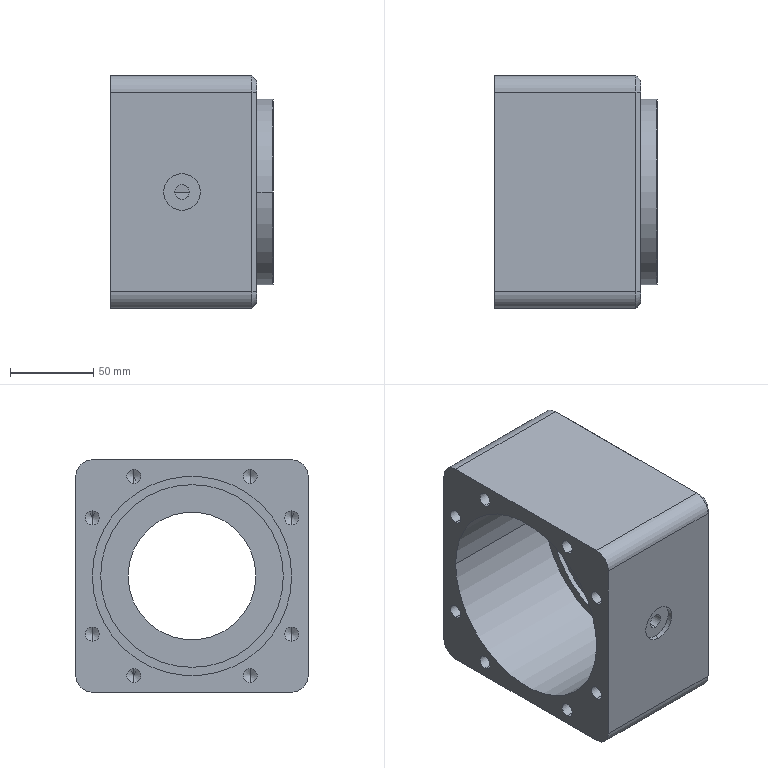Part | SolidWorks | features ICE 13, HoleWzd 7, Chamfer 4, MirrorPattern 4, CirPattern 1, Extrusion 1, Fillet 1 | 1 solid | 106 faces | box 98 x 140 x 140 mm | volume 787402 mm3 | cylinder 52 | cone 38 | plane 16 | commonest cylinder face diameters 8.5 x16 3.3 x8 14 x8 20 x4 8.8 x2 22 x2